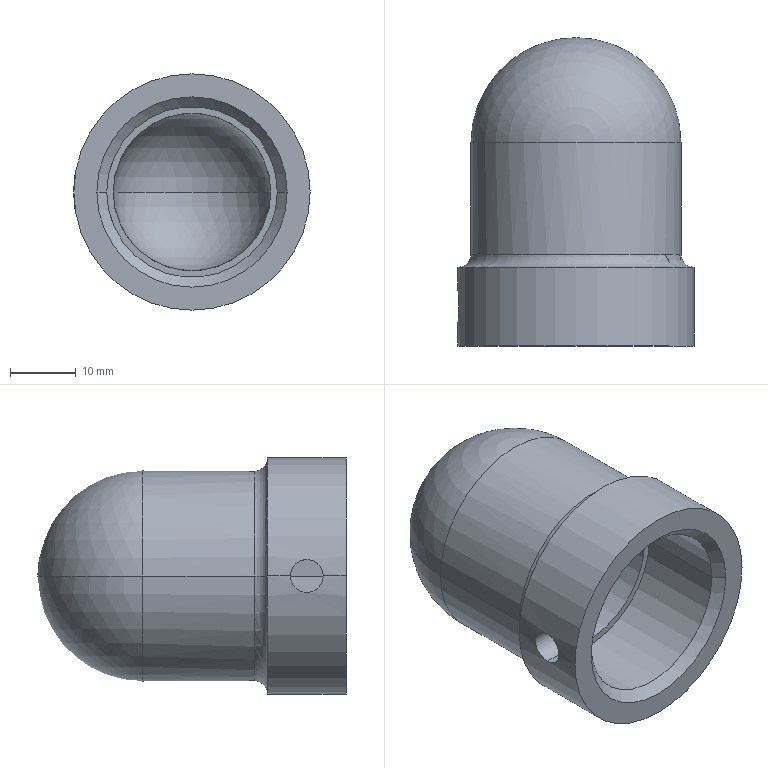Part | SolidWorks | features Chamfer 1, ICE 1, Revolution 1 | 1 solid | 20 faces | box 36 x 47 x 36 mm | volume 17147 mm3 | cylinder 10 | sphere 4 | cone 2 | torus 2 | plane 2 | commonest cylinder face diameters 5 x2 24 x2 26 x2 32 x2 36 x2
STEP:
#1=CARTESIAN_POINT('',(-13.,1.5,0.));
#2=VERTEX_POINT('',#1);
#3=CARTESIAN_POINT('',(13.,1.5,0.));
#4=VERTEX_POINT('',#3);
#5=CARTESIAN_POINT('',(0.,1.5,0.));
#6=DIRECTION('',(0.,-1.,0.));
#7=DIRECTION('',(-1.,0.,0.));
#8=AXIS2_PLACEMENT_3D('',#5,#6,#7);
#9=CIRCLE('',#8,13.);
#10=EDGE_CURVE('',#2,#4,#9,.T.);
#11=ORIENTED_EDGE('',*,*,#10,.F.);
#12=CARTESIAN_POINT('',(-14.5,0.,0.));
#13=VERTEX_POINT('',#12);
#14=CARTESIAN_POINT('',(-13.,1.5,0.));
#15=DIRECTION('',(-0.7071,-0.7071,0.));
#16=VECTOR('',#15,1000.);
#17=LINE('',#14,#16);
#18=EDGE_CURVE('',#2,#13,#17,.T.);
#19=ORIENTED_EDGE('',*,*,#18,.T.);
#20=CARTESIAN_POINT('',(14.5,0.,0.));
#21=VERTEX_POINT('',#20);
#22=CARTESIAN_POINT('',(0.,0.,0.));
#23=DIRECTION('',(0.,1.,0.));
#24=DIRECTION('',(-1.,0.,0.));
#25=AXIS2_PLACEMENT_3D('',#22,#23,#24);
#26=CIRCLE('',#25,14.5);
#27=EDGE_CURVE('',#21,#13,#26,.T.);
#28=ORIENTED_EDGE('',*,*,#27,.F.);
#29=CARTESIAN_POINT('',(13.,1.5,0.));
#30=DIRECTION('',(0.7071,-0.7071,0.));
#31=VECTOR('',#30,1000.);
#32=LINE('',#29,#31);
#33=EDGE_CURVE('',#4,#21,#32,.T.);
#34=ORIENTED_EDGE('',*,*,#33,.F.);
#35=EDGE_LOOP('',(#11,#19,#28,#34));
#36=FACE_OUTER_BOUND('',#35,.T.);
#37=CARTESIAN_POINT('',(0.,1.5,0.));
#38=DIRECTION('',(0.,-1.,0.));
#39=DIRECTION('',(1.,0.,0.));
#40=AXIS2_PLACEMENT_3D('',#37,#38,#39);
#41=CONICAL_SURFACE('',#40,13.,0.7854);
#42=ADVANCED_FACE('',(#36),#41,.F.);
#43=CARTESIAN_POINT('',(-17.826,6.,2.5));
#44=VERTEX_POINT('',#43);
#45=CARTESIAN_POINT('',(-18.,3.5,0.));
#46=VERTEX_POINT('',#45);
#47=CARTESIAN_POINT('',(-17.826,6.,2.5));
#48=CARTESIAN_POINT('',(-17.826,5.837,2.5));
#49=CARTESIAN_POINT('',(-17.828,5.674,2.484));
#50=CARTESIAN_POINT('',(-17.837,5.351,2.42));
#51=CARTESIAN_POINT('',(-17.843,5.194,2.372));
#52=CARTESIAN_POINT('',(-17.859,4.893,2.247));
#53=CARTESIAN_POINT('',(-17.869,4.747,2.169));
#54=CARTESIAN_POINT('',(-17.89,4.474,1.987));
#55=CARTESIAN_POINT('',(-17.902,4.348,1.884));
#56=CARTESIAN_POINT('',(-17.924,4.118,1.653));
#57=CARTESIAN_POINT('',(-17.936,4.012,1.525));
#58=CARTESIAN_POINT('',(-17.957,3.831,1.253));
#59=CARTESIAN_POINT('',(-17.966,3.754,1.11));
#60=CARTESIAN_POINT('',(-17.983,3.628,0.8067));
#61=CARTESIAN_POINT('',(-17.989,3.58,0.648));
#62=CARTESIAN_POINT('',(-17.998,3.516,0.3282));
#63=CARTESIAN_POINT('',(-18.,3.5,0.1653));
#64=CARTESIAN_POINT('',(-18.,3.5,0.));
#65=B_SPLINE_CURVE_WITH_KNOTS('',3,(#47,#48,#49,#50,#51,#52,#53,#54,#55,#56,#57,#58,#59,#60,#61,#62,#63,#64),.UNSPECIFIED.,.F.,.F.,(4,2,2,2,2,2,2,2,4),(0.007826,0.008315,0.008804,0.009293,0.009782,0.01027,0.01076,0.01125,0.01174),.UNSPECIFIED.);
#66=EDGE_CURVE('',#44,#46,#65,.T.);
#67=ORIENTED_EDGE('',*,*,#66,.F.);
#68=CARTESIAN_POINT('',(-12.757,6.,2.5));
#69=VERTEX_POINT('',#68);
#70=CARTESIAN_POINT('',(-40.,6.,2.5));
#71=DIRECTION('',(1.,0.,0.));
#72=VECTOR('',#71,1000.);
#73=LINE('',#70,#72);
#74=EDGE_CURVE('',#44,#69,#73,.T.);
#75=ORIENTED_EDGE('',*,*,#74,.T.);
#76=CARTESIAN_POINT('',(-13.,3.5,0.));
#77=VERTEX_POINT('',#76);
#78=CARTESIAN_POINT('',(-13.,3.5,0.));
#79=CARTESIAN_POINT('',(-13.,3.5,0.1635));
#80=CARTESIAN_POINT('',(-12.997,3.516,0.3295));
#81=CARTESIAN_POINT('',(-12.985,3.581,0.6504));
#82=CARTESIAN_POINT('',(-12.976,3.628,0.8063));
#83=CARTESIAN_POINT('',(-12.953,3.754,1.109));
#84=CARTESIAN_POINT('',(-12.94,3.832,1.255));
#85=CARTESIAN_POINT('',(-12.911,4.013,1.525));
#86=CARTESIAN_POINT('',(-12.895,4.116,1.652));
#87=CARTESIAN_POINT('',(-12.863,4.349,1.884));
#88=CARTESIAN_POINT('',(-12.847,4.475,1.988));
#89=CARTESIAN_POINT('',(-12.818,4.745,2.168));
#90=CARTESIAN_POINT('',(-12.805,4.892,2.247));
#91=CARTESIAN_POINT('',(-12.782,5.194,2.372));
#92=CARTESIAN_POINT('',(-12.773,5.35,2.419));
#93=CARTESIAN_POINT('',(-12.761,5.671,2.484));
#94=CARTESIAN_POINT('',(-12.757,5.837,2.5));
#95=CARTESIAN_POINT('',(-12.757,6.,2.5));
#96=B_SPLINE_CURVE_WITH_KNOTS('',3,(#78,#79,#80,#81,#82,#83,#84,#85,#86,#87,#88,#89,#90,#91,#92,#93,#94,#95),.UNSPECIFIED.,.F.,.F.,(4,2,2,2,2,2,2,2,4),(0.003918,0.004408,0.004897,0.005387,0.005876,0.006366,0.006855,0.007345,0.007834),.UNSPECIFIED.);
#97=EDGE_CURVE('',#77,#69,#96,.T.);
#98=ORIENTED_EDGE('',*,*,#97,.F.);
#99=CARTESIAN_POINT('',(-12.757,6.,-2.5));
#100=VERTEX_POINT('',#99);
#101=CARTESIAN_POINT('',(-12.757,6.,-2.5));
#102=CARTESIAN_POINT('',(-12.757,5.834,-2.5));
#103=CARTESIAN_POINT('',(-12.761,5.672,-2.484));
#104=CARTESIAN_POINT('',(-12.773,5.351,-2.42));
#105=CARTESIAN_POINT('',(-12.782,5.192,-2.372));
#106=CARTESIAN_POINT('',(-12.805,4.89,-2.246));
#107=CARTESIAN_POINT('',(-12.818,4.746,-2.169));
#108=CARTESIAN_POINT('',(-12.847,4.475,-1.988));
#109=CARTESIAN_POINT('',(-12.864,4.347,-1.882));
#110=CARTESIAN_POINT('',(-12.911,4.001,-1.537));
#111=CARTESIAN_POINT('',(-12.942,3.815,-1.258));
#112=CARTESIAN_POINT('',(-12.976,3.628,-0.8071));
#113=CARTESIAN_POINT('',(-12.985,3.58,-0.6491));
#114=CARTESIAN_POINT('',(-12.997,3.516,-0.3261));
#115=CARTESIAN_POINT('',(-13.,3.5,-0.1635));
#116=CARTESIAN_POINT('',(-13.,3.5,0.));
#117=B_SPLINE_CURVE_WITH_KNOTS('',3,(#101,#102,#103,#104,#105,#106,#107,#108,#109,#110,#111,#112,#113,#114,#115,#116),.UNSPECIFIED.,.F.,.F.,(4,2,2,2,2,2,2,4),(0.,0.0004898,0.0009795,0.001469,0.001959,0.002939,0.003428,0.003918),.UNSPECIFIED.);
#118=EDGE_CURVE('',#100,#77,#117,.T.);
#119=ORIENTED_EDGE('',*,*,#118,.F.);
#120=CARTESIAN_POINT('',(-17.826,6.,-2.5));
#121=VERTEX_POINT('',#120);
#122=CARTESIAN_POINT('',(-40.,6.,-2.5));
#123=DIRECTION('',(1.,0.,0.));
#124=VECTOR('',#123,1000.);
#125=LINE('',#122,#124);
#126=EDGE_CURVE('',#121,#100,#125,.T.);
#127=ORIENTED_EDGE('',*,*,#126,.F.);
#128=CARTESIAN_POINT('',(-18.,3.5,0.));
#129=CARTESIAN_POINT('',(-18.,3.5,-0.1652));
#130=CARTESIAN_POINT('',(-17.998,3.516,-0.3276));
#131=CARTESIAN_POINT('',(-17.989,3.58,-0.6473));
#132=CARTESIAN_POINT('',(-17.983,3.628,-0.8062));
#133=CARTESIAN_POINT('',(-17.966,3.753,-1.109));
#134=CARTESIAN_POINT('',(-17.957,3.83,-1.252));
#135=CARTESIAN_POINT('',(-17.936,4.011,-1.524));
#136=CARTESIAN_POINT('',(-17.924,4.117,-1.652));
#137=CARTESIAN_POINT('',(-17.89,4.462,-1.997));
#138=CARTESIAN_POINT('',(-17.867,4.74,-2.184));
#139=CARTESIAN_POINT('',(-17.835,5.341,-2.433));
#140=CARTESIAN_POINT('',(-17.826,5.669,-2.5));
#141=CARTESIAN_POINT('',(-17.826,6.,-2.5));
#142=B_SPLINE_CURVE_WITH_KNOTS('',3,(#128,#129,#130,#131,#132,#133,#134,#135,#136,#137,#138,#139,#140,#141),.UNSPECIFIED.,.F.,.F.,(4,2,2,2,2,2,4),(0.01174,0.01223,0.01272,0.01321,0.01369,0.01467,0.01565),.UNSPECIFIED.);
#143=EDGE_CURVE('',#46,#121,#142,.T.);
#144=ORIENTED_EDGE('',*,*,#143,.F.);
#145=EDGE_LOOP('',(#67,#75,#98,#119,#127,#144));
#146=FACE_OUTER_BOUND('',#145,.T.);
#147=CARTESIAN_POINT('',(-40.,6.,0.));
#148=DIRECTION('',(1.,0.,0.));
#149=DIRECTION('',(0.,0.,-1.));
#150=AXIS2_PLACEMENT_3D('',#147,#148,#149);
#151=CYLINDRICAL_SURFACE('',#150,2.5);
#152=ADVANCED_FACE('',(#146),#151,.F.);
#153=CARTESIAN_POINT('',(-12.,31.,0.));
#154=VERTEX_POINT('',#153);
#155=CARTESIAN_POINT('',(12.,31.,0.));
#156=VERTEX_POINT('',#155);
#157=CARTESIAN_POINT('',(0.,31.,0.));
#158=DIRECTION('',(0.,-1.,0.));
#159=DIRECTION('',(1.,0.,0.));
#160=AXIS2_PLACEMENT_3D('',#157,#158,#159);
#161=CIRCLE('',#160,12.);
#162=EDGE_CURVE('',#154,#156,#161,.T.);
#163=ORIENTED_EDGE('',*,*,#162,.F.);
#164=CARTESIAN_POINT('',(-12.,15.,0.));
#165=VERTEX_POINT('',#164);
#166=CARTESIAN_POINT('',(-12.,-51.943,0.));
#167=DIRECTION('',(0.,-1.,0.));
#168=VECTOR('',#167,1000.);
#169=LINE('',#166,#168);
#170=EDGE_CURVE('',#154,#165,#169,.T.);
#171=ORIENTED_EDGE('',*,*,#170,.T.);
#172=CARTESIAN_POINT('',(12.,15.,0.));
#173=VERTEX_POINT('',#172);
#174=CARTESIAN_POINT('',(0.,15.,0.));
#175=DIRECTION('',(0.,-1.,0.));
#176=DIRECTION('',(1.,0.,0.));
#177=AXIS2_PLACEMENT_3D('',#174,#175,#176);
#178=CIRCLE('',#177,12.);
#179=EDGE_CURVE('',#165,#173,#178,.T.);
#180=ORIENTED_EDGE('',*,*,#179,.T.);
#181=CARTESIAN_POINT('',(12.,-51.943,0.));
#182=DIRECTION('',(0.,-1.,0.));
#183=VECTOR('',#182,1000.);
#184=LINE('',#181,#183);
#185=EDGE_CURVE('',#156,#173,#184,.T.);
#186=ORIENTED_EDGE('',*,*,#185,.F.);
#187=EDGE_LOOP('',(#163,#171,#180,#186));
#188=FACE_OUTER_BOUND('',#187,.T.);
#189=CARTESIAN_POINT('',(0.,-51.943,0.));
#190=DIRECTION('',(0.,-1.,0.));
#191=DIRECTION('',(1.,0.,0.));
#192=AXIS2_PLACEMENT_3D('',#189,#190,#191);
#193=CYLINDRICAL_SURFACE('',#192,12.);
#194=ADVANCED_FACE('',(#188),#193,.F.);
#195=CARTESIAN_POINT('',(-13.,15.,0.));
#196=VERTEX_POINT('',#195);
#197=CARTESIAN_POINT('',(13.,15.,0.));
#198=VERTEX_POINT('',#197);
#199=CARTESIAN_POINT('',(0.,15.,0.));
#200=DIRECTION('',(0.,-1.,0.));
#201=DIRECTION('',(1.,0.,0.));
#202=AXIS2_PLACEMENT_3D('',#199,#200,#201);
#203=CIRCLE('',#202,13.);
#204=EDGE_CURVE('',#196,#198,#203,.T.);
#205=ORIENTED_EDGE('',*,*,#204,.F.);
#206=CARTESIAN_POINT('',(-13.,8.5,0.));
#207=VERTEX_POINT('',#206);
#208=CARTESIAN_POINT('',(-13.,-51.943,0.));
#209=DIRECTION('',(0.,-1.,0.));
#210=VECTOR('',#209,1000.);
#211=LINE('',#208,#210);
#212=EDGE_CURVE('',#196,#207,#211,.T.);
#213=ORIENTED_EDGE('',*,*,#212,.T.);
#214=CARTESIAN_POINT('',(-13.,8.5,0.));
#215=CARTESIAN_POINT('',(-13.,8.5,-0.165));
#216=CARTESIAN_POINT('',(-12.997,8.484,-0.3275));
#217=CARTESIAN_POINT('',(-12.985,8.42,-0.6477));
#218=CARTESIAN_POINT('',(-12.976,8.372,-0.807));
#219=CARTESIAN_POINT('',(-12.954,8.247,-1.109));
#220=CARTESIAN_POINT('',(-12.94,8.17,-1.252));
#221=CARTESIAN_POINT('',(-12.911,7.988,-1.524));
#222=CARTESIAN_POINT('',(-12.895,7.883,-1.652));
#223=CARTESIAN_POINT('',(-12.848,7.539,-1.997));
#224=CARTESIAN_POINT('',(-12.816,7.261,-2.183));
#225=CARTESIAN_POINT('',(-12.782,6.81,-2.371));
#226=CARTESIAN_POINT('',(-12.773,6.651,-2.419));
#227=CARTESIAN_POINT('',(-12.761,6.329,-2.484));
#228=CARTESIAN_POINT('',(-12.757,6.166,-2.5));
#229=CARTESIAN_POINT('',(-12.757,6.,-2.5));
#230=B_SPLINE_CURVE_WITH_KNOTS('',3,(#214,#215,#216,#217,#218,#219,#220,#221,#222,#223,#224,#225,#226,#227,#228,#229),.UNSPECIFIED.,.F.,.F.,(4,2,2,2,2,2,2,4),(0.01175,0.01224,0.01273,0.01322,0.01371,0.01469,0.01518,0.01567),.UNSPECIFIED.);
#231=EDGE_CURVE('',#207,#100,#230,.T.);
#232=ORIENTED_EDGE('',*,*,#231,.T.);
#233=ORIENTED_EDGE('',*,*,#118,.T.);
#234=CARTESIAN_POINT('',(-13.,-51.943,0.));
#235=DIRECTION('',(0.,-1.,0.));
#236=VECTOR('',#235,1000.);
#237=LINE('',#234,#236);
#238=EDGE_CURVE('',#77,#2,#237,.T.);
#239=ORIENTED_EDGE('',*,*,#238,.T.);
#240=ORIENTED_EDGE('',*,*,#10,.T.);
#241=CARTESIAN_POINT('',(13.,-51.943,0.));
#242=DIRECTION('',(0.,-1.,0.));
#243=VECTOR('',#242,1000.);
#244=LINE('',#241,#243);
#245=EDGE_CURVE('',#198,#4,#244,.T.);
#246=ORIENTED_EDGE('',*,*,#245,.F.);
#247=EDGE_LOOP('',(#205,#213,#232,#233,#239,#240,#246));
#248=FACE_OUTER_BOUND('',#247,.T.);
#249=CARTESIAN_POINT('',(0.,-51.943,0.));
#250=DIRECTION('',(0.,-1.,0.));
#251=DIRECTION('',(1.,0.,0.));
#252=AXIS2_PLACEMENT_3D('',#249,#250,#251);
#253=CYLINDRICAL_SURFACE('',#252,13.);
#254=ADVANCED_FACE('',(#248),#253,.F.);
#255=CARTESIAN_POINT('',(18.,12.,0.));
#256=VERTEX_POINT('',#255);
#257=CARTESIAN_POINT('',(-18.,12.,0.));
#258=VERTEX_POINT('',#257);
#259=CARTESIAN_POINT('',(0.,12.,0.));
#260=DIRECTION('',(0.,-1.,0.));
#261=DIRECTION('',(1.,0.,0.));
#262=AXIS2_PLACEMENT_3D('',#259,#260,#261);
#263=CIRCLE('',#262,18.);
#264=EDGE_CURVE('',#256,#258,#263,.T.);
#265=ORIENTED_EDGE('',*,*,#264,.T.);
#266=CARTESIAN_POINT('',(-18.,8.5,0.));
#267=VERTEX_POINT('',#266);
#268=CARTESIAN_POINT('',(-18.,-51.943,0.));
#269=DIRECTION('',(0.,-1.,0.));
#270=VECTOR('',#269,1000.);
#271=LINE('',#268,#270);
#272=EDGE_CURVE('',#258,#267,#271,.T.);
#273=ORIENTED_EDGE('',*,*,#272,.T.);
#274=CARTESIAN_POINT('',(-18.,8.5,0.));
#275=CARTESIAN_POINT('',(-18.,8.5,0.1632));
#276=CARTESIAN_POINT('',(-17.998,8.484,0.3291));
#277=CARTESIAN_POINT('',(-17.989,8.42,0.6498));
#278=CARTESIAN_POINT('',(-17.983,8.372,0.8057));
#279=CARTESIAN_POINT('',(-17.966,8.247,1.109));
#280=CARTESIAN_POINT('',(-17.957,8.169,1.255));
#281=CARTESIAN_POINT('',(-17.936,7.988,1.525));
#282=CARTESIAN_POINT('',(-17.924,7.884,1.651));
#283=CARTESIAN_POINT('',(-17.901,7.651,1.884));
#284=CARTESIAN_POINT('',(-17.89,7.525,1.988));
#285=CARTESIAN_POINT('',(-17.869,7.254,2.169));
#286=CARTESIAN_POINT('',(-17.859,7.108,2.247));
#287=CARTESIAN_POINT('',(-17.843,6.806,2.372));
#288=CARTESIAN_POINT('',(-17.837,6.65,2.42));
#289=CARTESIAN_POINT('',(-17.828,6.329,2.484));
#290=CARTESIAN_POINT('',(-17.826,6.163,2.5));
#291=CARTESIAN_POINT('',(-17.826,6.,2.5));
#292=B_SPLINE_CURVE_WITH_KNOTS('',3,(#274,#275,#276,#277,#278,#279,#280,#281,#282,#283,#284,#285,#286,#287,#288,#289,#290,#291),.UNSPECIFIED.,.F.,.F.,(4,2,2,2,2,2,2,2,4),(0.003914,0.004403,0.004892,0.005381,0.00587,0.006359,0.006848,0.007337,0.007826),.UNSPECIFIED.);
#293=EDGE_CURVE('',#267,#44,#292,.T.);
#294=ORIENTED_EDGE('',*,*,#293,.T.);
#295=ORIENTED_EDGE('',*,*,#66,.T.);
#296=CARTESIAN_POINT('',(-18.,0.,0.));
#297=VERTEX_POINT('',#296);
#298=CARTESIAN_POINT('',(-18.,-51.943,0.));
#299=DIRECTION('',(0.,-1.,0.));
#300=VECTOR('',#299,1000.);
#301=LINE('',#298,#300);
#302=EDGE_CURVE('',#46,#297,#301,.T.);
#303=ORIENTED_EDGE('',*,*,#302,.T.);
#304=CARTESIAN_POINT('',(18.,0.,0.));
#305=VERTEX_POINT('',#304);
#306=CARTESIAN_POINT('',(0.,0.,0.));
#307=DIRECTION('',(0.,-1.,0.));
#308=DIRECTION('',(1.,0.,0.));
#309=AXIS2_PLACEMENT_3D('',#306,#307,#308);
#310=CIRCLE('',#309,18.);
#311=EDGE_CURVE('',#305,#297,#310,.T.);
#312=ORIENTED_EDGE('',*,*,#311,.F.);
#313=CARTESIAN_POINT('',(18.,-51.943,0.));
#314=DIRECTION('',(0.,-1.,0.));
#315=VECTOR('',#314,1000.);
#316=LINE('',#313,#315);
#317=EDGE_CURVE('',#256,#305,#316,.T.);
#318=ORIENTED_EDGE('',*,*,#317,.F.);
#319=EDGE_LOOP('',(#265,#273,#294,#295,#303,#312,#318));
#320=FACE_OUTER_BOUND('',#319,.T.);
#321=CARTESIAN_POINT('',(0.,-51.943,0.));
#322=DIRECTION('',(0.,-1.,0.));
#323=DIRECTION('',(1.,0.,0.));
#324=AXIS2_PLACEMENT_3D('',#321,#322,#323);
#325=CYLINDRICAL_SURFACE('',#324,18.);
#326=ADVANCED_FACE('',(#320),#325,.T.);
#327=CARTESIAN_POINT('',(0.,12.,0.));
#328=DIRECTION('',(0.,-1.,0.));
#329=DIRECTION('',(1.,0.,0.));
#330=AXIS2_PLACEMENT_3D('',#327,#328,#329);
#331=CIRCLE('',#330,18.);
#332=EDGE_CURVE('',#258,#256,#331,.T.);
#333=ORIENTED_EDGE('',*,*,#332,.F.);
#334=CARTESIAN_POINT('',(-16.,14.,0.));
#335=VERTEX_POINT('',#334);
#336=CARTESIAN_POINT('',(-18.,14.,0.));
#337=DIRECTION('',(0.,0.,1.));
#338=DIRECTION('',(1.,0.,0.));
#339=AXIS2_PLACEMENT_3D('',#336,#337,#338);
#340=CIRCLE('',#339,2.);
#341=EDGE_CURVE('',#258,#335,#340,.T.);
#342=ORIENTED_EDGE('',*,*,#341,.T.);
#343=CARTESIAN_POINT('',(16.,14.,0.));
#344=VERTEX_POINT('',#343);
#345=CARTESIAN_POINT('',(0.,14.,0.));
#346=DIRECTION('',(0.,-1.,0.));
#347=DIRECTION('',(1.,0.,0.));
#348=AXIS2_PLACEMENT_3D('',#345,#346,#347);
#349=CIRCLE('',#348,16.);
#350=EDGE_CURVE('',#335,#344,#349,.T.);
#351=ORIENTED_EDGE('',*,*,#350,.T.);
#352=CARTESIAN_POINT('',(18.,14.,0.));
#353=DIRECTION('',(0.,0.,-1.));
#354=DIRECTION('',(-1.,0.,0.));
#355=AXIS2_PLACEMENT_3D('',#352,#353,#354);
#356=CIRCLE('',#355,2.);
#357=EDGE_CURVE('',#256,#344,#356,.T.);
#358=ORIENTED_EDGE('',*,*,#357,.F.);
#359=EDGE_LOOP('',(#333,#342,#351,#358));
#360=FACE_OUTER_BOUND('',#359,.T.);
#361=CARTESIAN_POINT('',(0.,14.,0.));
#362=DIRECTION('',(0.,-1.,0.));
#363=DIRECTION('',(1.,0.,0.));
#364=AXIS2_PLACEMENT_3D('',#361,#362,#363);
#365=TOROIDAL_SURFACE('',#364,18.,2.);
#366=ADVANCED_FACE('',(#360),#365,.F.);
#367=CARTESIAN_POINT('',(16.,31.,0.));
#368=VERTEX_POINT('',#367);
#369=CARTESIAN_POINT('',(-16.,31.,0.));
#370=VERTEX_POINT('',#369);
#371=CARTESIAN_POINT('',(0.,31.,0.));
#372=DIRECTION('',(0.,-1.,0.));
#373=DIRECTION('',(1.,0.,0.));
#374=AXIS2_PLACEMENT_3D('',#371,#372,#373);
#375=CIRCLE('',#374,16.);
#376=EDGE_CURVE('',#368,#370,#375,.T.);
#377=ORIENTED_EDGE('',*,*,#376,.T.);
#378=CARTESIAN_POINT('',(-16.,-51.943,0.));
#379=DIRECTION('',(0.,-1.,0.));
#380=VECTOR('',#379,1000.);
#381=LINE('',#378,#380);
#382=EDGE_CURVE('',#370,#335,#381,.T.);
#383=ORIENTED_EDGE('',*,*,#382,.T.);
#384=CARTESIAN_POINT('',(0.,14.,0.));
#385=DIRECTION('',(0.,-1.,0.));
#386=DIRECTION('',(1.,0.,0.));
#387=AXIS2_PLACEMENT_3D('',#384,#385,#386);
#388=CIRCLE('',#387,16.);
#389=EDGE_CURVE('',#344,#335,#388,.T.);
#390=ORIENTED_EDGE('',*,*,#389,.F.);
#391=CARTESIAN_POINT('',(16.,-51.943,0.));
#392=DIRECTION('',(0.,-1.,0.));
#393=VECTOR('',#392,1000.);
#394=LINE('',#391,#393);
#395=EDGE_CURVE('',#368,#344,#394,.T.);
#396=ORIENTED_EDGE('',*,*,#395,.F.);
#397=EDGE_LOOP('',(#377,#383,#390,#396));
#398=FACE_OUTER_BOUND('',#397,.T.);
#399=CARTESIAN_POINT('',(0.,-51.943,0.));
#400=DIRECTION('',(0.,-1.,0.));
#401=DIRECTION('',(1.,0.,0.));
#402=AXIS2_PLACEMENT_3D('',#399,#400,#401);
#403=CYLINDRICAL_SURFACE('',#402,16.);
#404=ADVANCED_FACE('',(#398),#403,.T.);
#405=CARTESIAN_POINT('',(0.,47.,0.));
#406=VERTEX_POINT('',#405);
#407=CARTESIAN_POINT('',(0.,31.,0.));
#408=DIRECTION('',(0.,0.,-1.));
#409=DIRECTION('',(-1.,0.,0.));
#410=AXIS2_PLACEMENT_3D('',#407,#408,#409);
#411=CIRCLE('',#410,16.);
#412=EDGE_CURVE('',#406,#368,#411,.T.);
#413=ORIENTED_EDGE('',*,*,#412,.F.);
#414=CARTESIAN_POINT('',(0.,31.,0.));
#415=DIRECTION('',(0.,0.,1.));
#416=DIRECTION('',(1.,0.,0.));
#417=AXIS2_PLACEMENT_3D('',#414,#415,#416);
#418=CIRCLE('',#417,16.);
#419=EDGE_CURVE('',#406,#370,#418,.T.);
#420=ORIENTED_EDGE('',*,*,#419,.T.);
#421=ORIENTED_EDGE('',*,*,#376,.F.);
#422=EDGE_LOOP('',(#413,#420,#421));
#423=FACE_OUTER_BOUND('',#422,.T.);
#424=CARTESIAN_POINT('',(0.,31.,0.));
#425=DIRECTION('',(0.,0.,1.));
#426=DIRECTION('',(1.,0.,0.));
#427=AXIS2_PLACEMENT_3D('',#424,#425,#426);
#428=SPHERICAL_SURFACE('',#427,16.);
#429=ADVANCED_FACE('',(#423),#428,.T.);
#430=CARTESIAN_POINT('',(0.,43.,0.));
#431=VERTEX_POINT('',#430);
#432=CARTESIAN_POINT('',(0.,31.,0.));
#433=DIRECTION('',(0.,0.,1.));
#434=DIRECTION('',(1.,0.,0.));
#435=AXIS2_PLACEMENT_3D('',#432,#433,#434);
#436=CIRCLE('',#435,12.);
#437=EDGE_CURVE('',#431,#154,#436,.T.);
#438=ORIENTED_EDGE('',*,*,#437,.F.);
#439=CARTESIAN_POINT('',(0.,31.,0.));
#440=DIRECTION('',(0.,0.,-1.));
#441=DIRECTION('',(-1.,0.,0.));
#442=AXIS2_PLACEMENT_3D('',#439,#440,#441);
#443=CIRCLE('',#442,12.);
#444=EDGE_CURVE('',#431,#156,#443,.T.);
#445=ORIENTED_EDGE('',*,*,#444,.T.);
#446=CARTESIAN_POINT('',(0.,31.,0.));
#447=DIRECTION('',(0.,-1.,0.));
#448=DIRECTION('',(1.,0.,0.));
#449=AXIS2_PLACEMENT_3D('',#446,#447,#448);
#450=CIRCLE('',#449,12.);
#451=EDGE_CURVE('',#156,#154,#450,.T.);
#452=ORIENTED_EDGE('',*,*,#451,.T.);
#453=EDGE_LOOP('',(#438,#445,#452));
#454=FACE_OUTER_BOUND('',#453,.T.);
#455=CARTESIAN_POINT('',(0.,31.,0.));
#456=DIRECTION('',(0.,0.,-1.));
#457=DIRECTION('',(-1.,0.,0.));
#458=AXIS2_PLACEMENT_3D('',#455,#456,#457);
#459=SPHERICAL_SURFACE('',#458,12.);
#460=ADVANCED_FACE('',(#454),#459,.F.);
#461=ORIENTED_EDGE('',*,*,#444,.F.);
#462=ORIENTED_EDGE('',*,*,#437,.T.);
#463=ORIENTED_EDGE('',*,*,#162,.T.);
#464=EDGE_LOOP('',(#461,#462,#463));
#465=FACE_OUTER_BOUND('',#464,.T.);
#466=CARTESIAN_POINT('',(0.,31.,0.));
#467=DIRECTION('',(0.,0.,-1.));
#468=DIRECTION('',(-1.,0.,0.));
#469=AXIS2_PLACEMENT_3D('',#466,#467,#468);
#470=SPHERICAL_SURFACE('',#469,12.);
#471=ADVANCED_FACE('',(#465),#470,.F.);
#472=ORIENTED_EDGE('',*,*,#419,.F.);
#473=ORIENTED_EDGE('',*,*,#412,.T.);
#474=CARTESIAN_POINT('',(0.,31.,0.));
#475=DIRECTION('',(0.,-1.,0.));
#476=DIRECTION('',(1.,0.,0.));
#477=AXIS2_PLACEMENT_3D('',#474,#475,#476);
#478=CIRCLE('',#477,16.);
#479=EDGE_CURVE('',#370,#368,#478,.T.);
#480=ORIENTED_EDGE('',*,*,#479,.F.);
#481=EDGE_LOOP('',(#472,#473,#480));
#482=FACE_OUTER_BOUND('',#481,.T.);
#483=CARTESIAN_POINT('',(0.,31.,0.));
#484=DIRECTION('',(0.,0.,1.));
#485=DIRECTION('',(1.,0.,0.));
#486=AXIS2_PLACEMENT_3D('',#483,#484,#485);
#487=SPHERICAL_SURFACE('',#486,16.);
#488=ADVANCED_FACE('',(#482),#487,.T.);
#489=ORIENTED_EDGE('',*,*,#382,.F.);
#490=ORIENTED_EDGE('',*,*,#479,.T.);
#491=ORIENTED_EDGE('',*,*,#395,.T.);
#492=ORIENTED_EDGE('',*,*,#350,.F.);
#493=EDGE_LOOP('',(#489,#490,#491,#492));
#494=FACE_OUTER_BOUND('',#493,.T.);
#495=CARTESIAN_POINT('',(0.,-51.943,0.));
#496=DIRECTION('',(0.,-1.,0.));
#497=DIRECTION('',(1.,0.,0.));
#498=AXIS2_PLACEMENT_3D('',#495,#496,#497);
#499=CYLINDRICAL_SURFACE('',#498,16.);
#500=ADVANCED_FACE('',(#494),#499,.T.);
#501=ORIENTED_EDGE('',*,*,#341,.F.);
#502=ORIENTED_EDGE('',*,*,#264,.F.);
#503=ORIENTED_EDGE('',*,*,#357,.T.);
#504=ORIENTED_EDGE('',*,*,#389,.T.);
#505=EDGE_LOOP('',(#501,#502,#503,#504));
#506=FACE_OUTER_BOUND('',#505,.T.);
#507=CARTESIAN_POINT('',(0.,14.,0.));
#508=DIRECTION('',(0.,-1.,0.));
#509=DIRECTION('',(1.,0.,0.));
#510=AXIS2_PLACEMENT_3D('',#507,#508,#509);
#511=TOROIDAL_SURFACE('',#510,18.,2.);
#512=ADVANCED_FACE('',(#506),#511,.F.);
#513=ORIENTED_EDGE('',*,*,#272,.F.);
#514=ORIENTED_EDGE('',*,*,#332,.T.);
#515=ORIENTED_EDGE('',*,*,#317,.T.);
#516=CARTESIAN_POINT('',(0.,0.,0.));
#517=DIRECTION('',(0.,-1.,0.));
#518=DIRECTION('',(1.,0.,0.));
#519=AXIS2_PLACEMENT_3D('',#516,#517,#518);
#520=CIRCLE('',#519,18.);
#521=EDGE_CURVE('',#297,#305,#520,.T.);
#522=ORIENTED_EDGE('',*,*,#521,.F.);
#523=ORIENTED_EDGE('',*,*,#302,.F.);
#524=ORIENTED_EDGE('',*,*,#143,.T.);
#525=CARTESIAN_POINT('',(-17.826,6.,-2.5));
#526=CARTESIAN_POINT('',(-17.826,6.165,-2.5));
#527=CARTESIAN_POINT('',(-17.828,6.328,-2.484));
#528=CARTESIAN_POINT('',(-17.837,6.648,-2.42));
#529=CARTESIAN_POINT('',(-17.843,6.807,-2.372));
#530=CARTESIAN_POINT('',(-17.859,7.11,-2.246));
#531=CARTESIAN_POINT('',(-17.869,7.253,-2.169));
#532=CARTESIAN_POINT('',(-17.89,7.525,-1.988));
#533=CARTESIAN_POINT('',(-17.902,7.653,-1.882));
#534=CARTESIAN_POINT('',(-17.924,7.884,-1.652));
#535=CARTESIAN_POINT('',(-17.936,7.987,-1.526));
#536=CARTESIAN_POINT('',(-17.957,8.17,-1.253));
#537=CARTESIAN_POINT('',(-17.967,8.247,-1.107));
#538=CARTESIAN_POINT('',(-17.983,8.372,-0.8065));
#539=CARTESIAN_POINT('',(-17.989,8.42,-0.6486));
#540=CARTESIAN_POINT('',(-17.998,8.484,-0.3257));
#541=CARTESIAN_POINT('',(-18.,8.5,-0.1633));
#542=CARTESIAN_POINT('',(-18.,8.5,0.));
#543=B_SPLINE_CURVE_WITH_KNOTS('',3,(#525,#526,#527,#528,#529,#530,#531,#532,#533,#534,#535,#536,#537,#538,#539,#540,#541,#542),.UNSPECIFIED.,.F.,.F.,(4,2,2,2,2,2,2,2,4),(0.,0.0004892,0.0009784,0.001468,0.001957,0.002446,0.002935,0.003425,0.003914),.UNSPECIFIED.);
#544=EDGE_CURVE('',#121,#267,#543,.T.);
#545=ORIENTED_EDGE('',*,*,#544,.T.);
#546=EDGE_LOOP('',(#513,#514,#515,#522,#523,#524,#545));
#547=FACE_OUTER_BOUND('',#546,.T.);
#548=CARTESIAN_POINT('',(0.,-51.943,0.));
#549=DIRECTION('',(0.,-1.,0.));
#550=DIRECTION('',(1.,0.,0.));
#551=AXIS2_PLACEMENT_3D('',#548,#549,#550);
#552=CYLINDRICAL_SURFACE('',#551,18.);
#553=ADVANCED_FACE('',(#547),#552,.T.);
#554=ORIENTED_EDGE('',*,*,#27,.T.);
#555=CARTESIAN_POINT('',(0.,0.,0.));
#556=DIRECTION('',(0.,1.,0.));
#557=DIRECTION('',(-1.,0.,0.));
#558=AXIS2_PLACEMENT_3D('',#555,#556,#557);
#559=CIRCLE('',#558,14.5);
#560=EDGE_CURVE('',#13,#21,#559,.T.);
#561=ORIENTED_EDGE('',*,*,#560,.T.);
#562=EDGE_LOOP('',(#554,#561));
#563=FACE_BOUND('',#562,.T.);
#564=ORIENTED_EDGE('',*,*,#311,.T.);
#565=ORIENTED_EDGE('',*,*,#521,.T.);
#566=EDGE_LOOP('',(#564,#565));
#567=FACE_OUTER_BOUND('',#566,.T.);
#568=CARTESIAN_POINT('',(-13.,0.,0.));
#569=DIRECTION('',(0.,1.,0.));
#570=DIRECTION('',(-1.,0.,0.));
#571=AXIS2_PLACEMENT_3D('',#568,#569,#570);
#572=PLANE('',#571);
#573=ADVANCED_FACE('',(#563,#567),#572,.F.);
#574=ORIENTED_EDGE('',*,*,#212,.F.);
#575=CARTESIAN_POINT('',(0.,15.,0.));
#576=DIRECTION('',(0.,-1.,0.));
#577=DIRECTION('',(1.,0.,0.));
#578=AXIS2_PLACEMENT_3D('',#575,#576,#577);
#579=CIRCLE('',#578,13.);
#580=EDGE_CURVE('',#198,#196,#579,.T.);
#581=ORIENTED_EDGE('',*,*,#580,.F.);
#582=ORIENTED_EDGE('',*,*,#245,.T.);
#583=CARTESIAN_POINT('',(0.,1.5,0.));
#584=DIRECTION('',(0.,-1.,0.));
#585=DIRECTION('',(-1.,0.,0.));
#586=AXIS2_PLACEMENT_3D('',#583,#584,#585);
#587=CIRCLE('',#586,13.);
#588=EDGE_CURVE('',#4,#2,#587,.T.);
#589=ORIENTED_EDGE('',*,*,#588,.T.);
#590=ORIENTED_EDGE('',*,*,#238,.F.);
#591=ORIENTED_EDGE('',*,*,#97,.T.);
#592=CARTESIAN_POINT('',(-12.757,6.,2.5));
#593=CARTESIAN_POINT('',(-12.757,6.327,2.5));
#594=CARTESIAN_POINT('',(-12.771,6.657,2.434));
#595=CARTESIAN_POINT('',(-12.805,7.108,2.247));
#596=CARTESIAN_POINT('',(-12.818,7.254,2.169));
#597=CARTESIAN_POINT('',(-12.848,7.526,1.987));
#598=CARTESIAN_POINT('',(-12.863,7.652,1.884));
#599=CARTESIAN_POINT('',(-12.895,7.882,1.653));
#600=CARTESIAN_POINT('',(-12.911,7.988,1.525));
#601=CARTESIAN_POINT('',(-12.94,8.169,1.254));
#602=CARTESIAN_POINT('',(-12.953,8.246,1.111));
#603=CARTESIAN_POINT('',(-12.976,8.372,0.8071));
#604=CARTESIAN_POINT('',(-12.985,8.42,0.6488));
#605=CARTESIAN_POINT('',(-12.997,8.484,0.329));
#606=CARTESIAN_POINT('',(-13.,8.5,0.1651));
#607=CARTESIAN_POINT('',(-13.,8.5,0.));
#608=B_SPLINE_CURVE_WITH_KNOTS('',3,(#592,#593,#594,#595,#596,#597,#598,#599,#600,#601,#602,#603,#604,#605,#606,#607),.UNSPECIFIED.,.F.,.F.,(4,2,2,2,2,2,2,4),(0.007834,0.008814,0.009303,0.009793,0.01028,0.01077,0.01126,0.01175),.UNSPECIFIED.);
#609=EDGE_CURVE('',#69,#207,#608,.T.);
#610=ORIENTED_EDGE('',*,*,#609,.T.);
#611=EDGE_LOOP('',(#574,#581,#582,#589,#590,#591,#610));
#612=FACE_OUTER_BOUND('',#611,.T.);
#613=CARTESIAN_POINT('',(0.,-51.943,0.));
#614=DIRECTION('',(0.,-1.,0.));
#615=DIRECTION('',(1.,0.,0.));
#616=AXIS2_PLACEMENT_3D('',#613,#614,#615);
#617=CYLINDRICAL_SURFACE('',#616,13.);
#618=ADVANCED_FACE('',(#612),#617,.F.);
#619=CARTESIAN_POINT('',(0.,15.,0.));
#620=DIRECTION('',(0.,-1.,0.));
#621=DIRECTION('',(1.,0.,0.));
#622=AXIS2_PLACEMENT_3D('',#619,#620,#621);
#623=CIRCLE('',#622,12.);
#624=EDGE_CURVE('',#173,#165,#623,.T.);
#625=ORIENTED_EDGE('',*,*,#624,.F.);
#626=ORIENTED_EDGE('',*,*,#179,.F.);
#627=EDGE_LOOP('',(#625,#626));
#628=FACE_BOUND('',#627,.T.);
#629=ORIENTED_EDGE('',*,*,#580,.T.);
#630=ORIENTED_EDGE('',*,*,#204,.T.);
#631=EDGE_LOOP('',(#629,#630));
#632=FACE_OUTER_BOUND('',#631,.T.);
#633=CARTESIAN_POINT('',(-12.,15.,0.));
#634=DIRECTION('',(0.,1.,0.));
#635=DIRECTION('',(-1.,0.,0.));
#636=AXIS2_PLACEMENT_3D('',#633,#634,#635);
#637=PLANE('',#636);
#638=ADVANCED_FACE('',(#628,#632),#637,.F.);
#639=ORIENTED_EDGE('',*,*,#170,.F.);
#640=ORIENTED_EDGE('',*,*,#451,.F.);
#641=ORIENTED_EDGE('',*,*,#185,.T.);
#642=ORIENTED_EDGE('',*,*,#624,.T.);
#643=EDGE_LOOP('',(#639,#640,#641,#642));
#644=FACE_OUTER_BOUND('',#643,.T.);
#645=CARTESIAN_POINT('',(0.,-51.943,0.));
#646=DIRECTION('',(0.,-1.,0.));
#647=DIRECTION('',(1.,0.,0.));
#648=AXIS2_PLACEMENT_3D('',#645,#646,#647);
#649=CYLINDRICAL_SURFACE('',#648,12.);
#650=ADVANCED_FACE('',(#644),#649,.F.);
#651=ORIENTED_EDGE('',*,*,#74,.F.);
#652=ORIENTED_EDGE('',*,*,#293,.F.);
#653=ORIENTED_EDGE('',*,*,#544,.F.);
#654=ORIENTED_EDGE('',*,*,#126,.T.);
#655=ORIENTED_EDGE('',*,*,#231,.F.);
#656=ORIENTED_EDGE('',*,*,#609,.F.);
#657=EDGE_LOOP('',(#651,#652,#653,#654,#655,#656));
#658=FACE_OUTER_BOUND('',#657,.T.);
#659=CARTESIAN_POINT('',(-40.,6.,0.));
#660=DIRECTION('',(1.,0.,0.));
#661=DIRECTION('',(0.,0.,-1.));
#662=AXIS2_PLACEMENT_3D('',#659,#660,#661);
#663=CYLINDRICAL_SURFACE('',#662,2.5);
#664=ADVANCED_FACE('',(#658),#663,.F.);
#665=ORIENTED_EDGE('',*,*,#18,.F.);
#666=ORIENTED_EDGE('',*,*,#588,.F.);
#667=ORIENTED_EDGE('',*,*,#33,.T.);
#668=ORIENTED_EDGE('',*,*,#560,.F.);
#669=EDGE_LOOP('',(#665,#666,#667,#668));
#670=FACE_OUTER_BOUND('',#669,.T.);
#671=CARTESIAN_POINT('',(0.,1.5,0.));
#672=DIRECTION('',(0.,-1.,0.));
#673=DIRECTION('',(1.,0.,0.));
#674=AXIS2_PLACEMENT_3D('',#671,#672,#673);
#675=CONICAL_SURFACE('',#674,13.,0.7854);
#676=ADVANCED_FACE('',(#670),#675,.F.);
#677=CLOSED_SHELL('',(#42,#152,#194,#254,#326,#366,#404,#429,#460,#471,#488,#500,#512,#553,#573,#618,#638,#650,#664,#676));
#678=MANIFOLD_SOLID_BREP('',#677);
#679=CARTESIAN_POINT('',(0.,0.,0.));
#680=DIRECTION('',(0.,0.,1.));
#681=DIRECTION('',(1.,0.,0.));
#682=AXIS2_PLACEMENT_3D('',#679,#680,#681);
#683=(LENGTH_UNIT()NAMED_UNIT(*)SI_UNIT(.MILLI.,.METRE.));
#684=UNCERTAINTY_MEASURE_WITH_UNIT(LENGTH_MEASURE(0.00001),#683,'','');
#685=(NAMED_UNIT(*)PLANE_ANGLE_UNIT()SI_UNIT($,.RADIAN.));
#686=(NAMED_UNIT(*)SI_UNIT($,.STERADIAN.)SOLID_ANGLE_UNIT());
#687=(GEOMETRIC_REPRESENTATION_CONTEXT(3)GLOBAL_UNCERTAINTY_ASSIGNED_CONTEXT((#684))GLOBAL_UNIT_ASSIGNED_CONTEXT((#683,#685,#686))REPRESENTATION_CONTEXT('',''));
#688=ADVANCED_BREP_SHAPE_REPRESENTATION('',(#678,#682),#687);